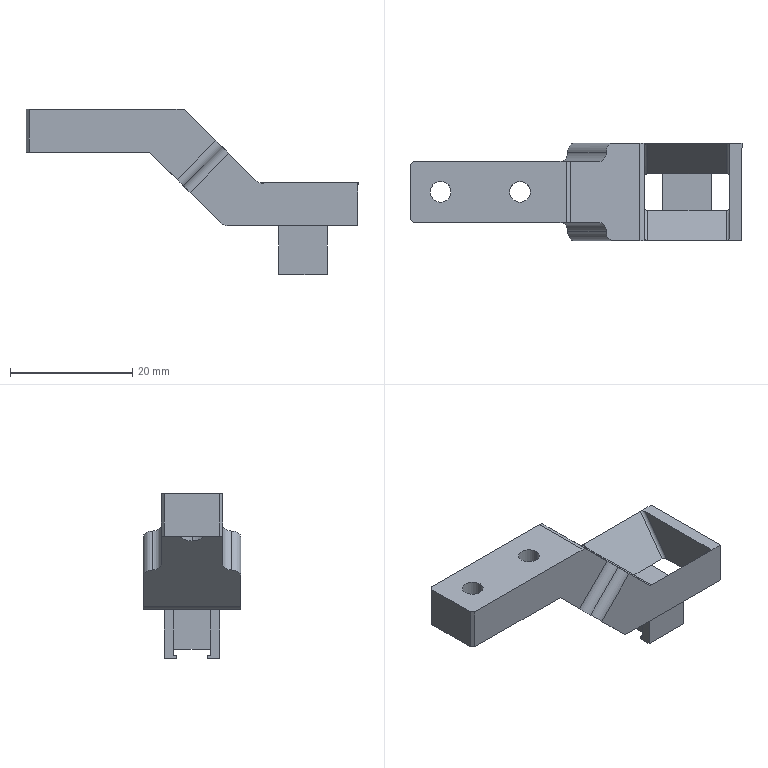NC program | NX | posted with a generic post | part box 54.3 x 16 x 27 mm
Lines 2093 to 2256 of 2256:
(HOLE_MILLING , TOOL : D4)
N4166 T04 M6
N4168 G54
N4170 G17 G0 G90 X-22.15 Y0. S9500 M3
N4172 G43 Z30. H4
N4174 Z-19.5
N4176 G94 G3 X-21.65 Y-0.5 R0.5 F1250.
N4178 X-21.15 Y0. R0.5
N4180 X-21.15 Y0. Z-19.8 I-1. J0.
N4182 X-21.15 Y0. Z-20.1 I-1. J0.
N4184 X-21.15 Y0. Z-20.4 I-1. J0.
N4186 X-21.15 Y0. Z-20.7 I-1. J0.
N4188 X-21.15 Y0. Z-21. I-1. J0.
N4190 X-21.15 Y0. Z-21.3 I-1. J0.
N4192 X-21.15 Y0. Z-21.6 I-1. J0.
N4194 X-21.15 Y0. Z-21.9 I-1. J0.
N4196 X-21.15 Y0. Z-22.2 I-1. J0.
N4198 X-21.15 Y0. Z-22.5 I-1. J0.
N4200 X-21.15 Y0. Z-22.8 I-1. J0.
N4202 X-21.15 Y0. Z-23.1 I-1. J0.
N4204 X-21.15 Y0. Z-23.4 I-1. J0.
N4206 X-22.15 Y1. R1.
N4208 X-21.15 Y0. R-1.
N4210 X-21.65 Y0.5 R0.5
N4212 X-22.15 Y0. R0.5
N4214 G0 Z30.
N4216 X-9.15
N4218 Z-18.736
N4220 G3 X-8.65 Y-0.5 R0.5
N4222 X-8.15 Y0. R0.5
N4224 X-8.15 Y0. Z-19.036 I-1. J0.
N4226 X-8.15 Y0. Z-19.336 I-1. J0.
N4228 X-8.15 Y0. Z-19.636 I-1. J0.
N4230 X-8.15 Y0. Z-19.936 I-1. J0.
N4232 X-8.15 Y0. Z-20.236 I-1. J0.
N4234 X-8.15 Y0. Z-20.536 I-1. J0.
N4236 X-8.15 Y0. Z-20.836 I-1. J0.
N4238 X-8.15 Y0. Z-21.136 I-1. J0.
N4240 X-8.15 Y0. Z-21.436 I-1. J0.
N4242 X-8.15 Y0. Z-21.736 I-1. J0.
N4244 X-8.15 Y0. Z-22.036 I-1. J0.
N4246 X-8.15 Y0. Z-22.336 I-1. J0.
N4248 X-8.15 Y0. Z-22.636 I-1. J0.
N4250 X-8.15 Y0. Z-22.936 I-1. J0.
N4252 X-8.15 Y0. Z-23.236 I-1. J0.
N4254 X-10.106 Y-0.293 Z-23.4 R-1.
N4256 X-8.857 Y-0.956 R1.
N4258 X-10.106 Y-0.293 R-1.
N4260 X-9.482 Y-0.624 R0.5
N4262 X-9.15 Y0. R0.5
N4264 G0 Z30.
N4266 M5
(ZLEVEL_PROFILE_1_COPY_1_COPY_1 , TOOL : D6A45)
N4268 T07 M6
N4270 G54
N4272 G17 G0 G90 X23.07 Y-6.451 S9500 M3
N4274 G43 Z30. H7
N4276 Z0.
N4278 G94 G1 Z-1. F1000.
N4280 X22.67 Y-5.759
N4282 G3 X22.151 Y-5.459 R0.6
N4284 G1 X14.149
N4286 G2 X13.191 Y-4.501 R0.958
N4288 G1 Y-2.499
N4290 G2 X14.149 Y-1.541 R0.958
N4292 G1 X22.151
N4294 G2 X23.109 Y-2.499 R0.958
N4296 G1 Y-4.501
N4298 G2 X22.151 Y-5.459 R0.964
N4300 G3 X21.633 Y-5.762 R0.6
N4302 G1 X21.122 Y-6.659
N4304 Z0.
N4306 G0 Z30.
N4308 X13.229 Y6.452
N4310 Z0.
N4312 G1 Z-1.
N4314 X13.63 Y5.759
N4316 G3 X14.149 Y5.459 R0.6
N4318 G1 X22.151
N4320 G2 X23.109 Y4.501 R0.964
N4322 G1 Y2.499
N4324 G2 X22.151 Y1.541 R0.958
N4326 G1 X14.149
N4328 G2 X13.191 Y2.499 R0.958
N4330 G1 Y4.501
N4332 G2 X14.149 Y5.459 R0.958
N4334 G3 X14.669 Y5.759 R0.6
N4336 G1 X15.188 Y6.659
N4338 Z0.
N4340 G0 Z30.
(ZLEVEL_PROFILE_1_COPY_1_COPY_1_COPY , TOOL : D6A45)
N4342 X5.343 Y10.181
N4344 Z-8.
N4346 G1 Z-9.
N4348 X5.588 Y9.369
N4350 G3 X6.025 Y8.959 R0.6
N4352 G1 X27.151
N4354 G2 X28.109 Y8.001 R0.958
N4356 G1 Y-8.001
N4358 G2 X27.151 Y-8.959 R0.958
N4360 G1 X6.038
N4362 G3 X5.603 Y-9.372 R0.6
N4364 G1 X5.363 Y-10.183
N4366 Z-8.
N4368 G0 Z30.
(ZLEVEL_PROFILE_1_COPY_1_COPY_1_COPY_COPY , TOOL : D6A45)
N4370 X-9.119 Y0.841
N4372 Z-20.
N4374 G1 Z-21.
N4376 X-8.105 Y1.713
N4378 X-8.13 Y1.762
N4380 X-8.17 Y1.798
N4382 X-8.221 Y1.818
N4384 G3 X-8.223 Y-1.819 R-2.041
N4386 G1 X-8.172 Y-1.799
N4388 X-8.132 Y-1.763
N4390 X-8.107 Y-1.715
N4392 X-9.119 Y-0.841
N4394 Z-20.
N4396 G0 Z30.
N4398 X-22.956 Y0.241
N4400 Z-20.
N4402 G1 Z-21.
N4404 X-23.891 Y0.52
N4406 G3 X-24.191 Y0. R0.6
N4408 G1 Y-0.003
N4410 G3 X-22.147 Y-2.041 R2.041
N4412 X-24.191 Y0. R-2.041
N4414 X-23.891 Y-0.52 R0.6
N4416 G1 X-22.956 Y-0.241
N4418 Z-20.
N4420 G0 Z30.
N4422 X-8.563 Y-7.159
N4424 Z-20.
N4426 G1 Z-21.
N4428 X-7.926 Y-5.999
N4430 X-7.97 Y-5.967
N4432 X-8.022 Y-5.953
N4434 X-8.076 Y-5.959
N4436 X-26.651
N4438 G2 X-27.327 Y-5.678 R0.957
N4440 G1 X-27.829 Y-5.177
N4442 G2 X-28.109 Y-4.501 R0.957
N4444 G1 Y4.501
N4446 G2 X-27.829 Y5.177 R0.957
N4448 G1 X-27.327 Y5.678
N4450 G2 X-26.651 Y5.959 R0.957
N4452 G1 X-8.076
N4454 X-8.022 Y5.953
N4456 X-7.97 Y5.967
N4458 X-7.926 Y5.999
N4460 X-8.563 Y7.159
N4462 Z-20.
N4464 G0 Z30.
N4466 M5
N4468 M2